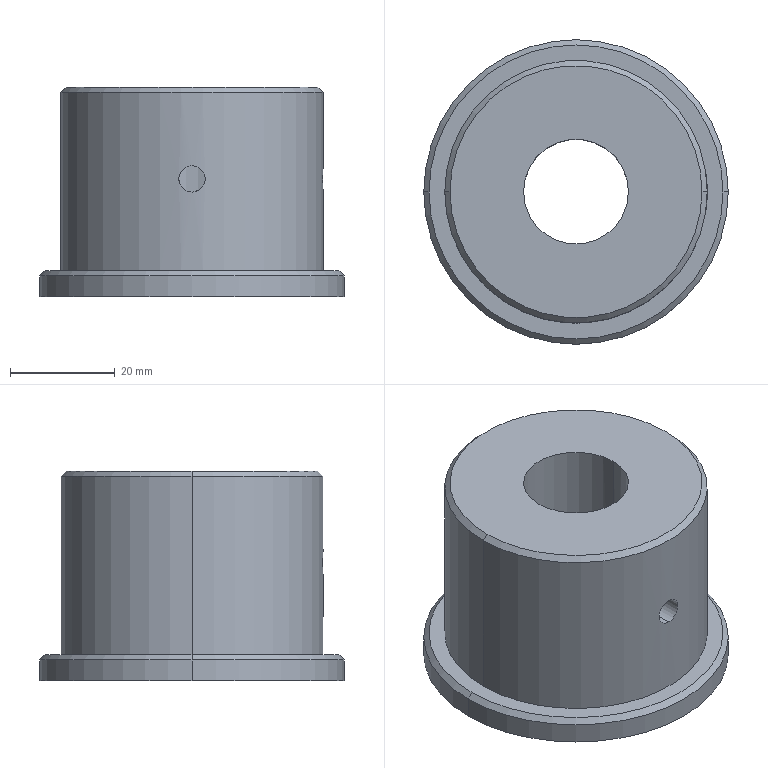Part | SolidWorks | features BaseBody 1 | 1 solid | 17 faces | box 58 x 58 x 40 mm | volume 68608 mm3 | cylinder 10 | cone 4 | plane 3 | commonest cylinder face diameters 5 x4 20 x2 50 x2 58 x2
STEP:
#1=CARTESIAN_POINT('',(24.875,2.5,22.5));
#2=VERTEX_POINT('',#1);
#3=CARTESIAN_POINT('',(25.,0.,20.));
#4=VERTEX_POINT('',#3);
#5=CARTESIAN_POINT('',(24.875,2.5,22.5));
#6=CARTESIAN_POINT('',(24.875,2.5,22.335));
#7=CARTESIAN_POINT('',(24.876,2.484,22.172));
#8=CARTESIAN_POINT('',(24.883,2.42,21.853));
#9=CARTESIAN_POINT('',(24.887,2.372,21.694));
#10=CARTESIAN_POINT('',(24.899,2.247,21.392));
#11=CARTESIAN_POINT('',(24.906,2.17,21.248));
#12=CARTESIAN_POINT('',(24.921,1.989,20.977));
#13=CARTESIAN_POINT('',(24.929,1.884,20.848));
#14=CARTESIAN_POINT('',(24.946,1.653,20.618));
#15=CARTESIAN_POINT('',(24.954,1.528,20.514));
#16=CARTESIAN_POINT('',(24.969,1.255,20.331));
#17=CARTESIAN_POINT('',(24.976,1.109,20.254));
#18=CARTESIAN_POINT('',(24.993,0.6586,20.066));
#19=CARTESIAN_POINT('',(25.,0.3304,20.));
#20=CARTESIAN_POINT('',(25.,0.,20.));
#21=B_SPLINE_CURVE_WITH_KNOTS('',3,(#5,#6,#7,#8,#9,#10,#11,#12,#13,#14,#15,#16,#17,#18,#19,#20),.UNSPECIFIED.,.F.,.F.,(4,2,2,2,2,2,2,4),(0.,0.0004885,0.000977,0.001465,0.001954,0.002442,0.002931,0.003908),.UNSPECIFIED.);
#22=EDGE_CURVE('',#2,#4,#21,.T.);
#23=ORIENTED_EDGE('',*,*,#22,.F.);
#24=CARTESIAN_POINT('',(9.682,2.5,22.5));
#25=VERTEX_POINT('',#24);
#26=CARTESIAN_POINT('',(29.,2.5,22.5));
#27=DIRECTION('',(-1.,0.,0.));
#28=VECTOR('',#27,1000.);
#29=LINE('',#26,#28);
#30=EDGE_CURVE('',#2,#25,#29,.T.);
#31=ORIENTED_EDGE('',*,*,#30,.T.);
#32=CARTESIAN_POINT('',(10.,0.,20.));
#33=VERTEX_POINT('',#32);
#34=CARTESIAN_POINT('',(9.682,2.5,22.5));
#35=CARTESIAN_POINT('',(9.682,2.5,22.334));
#36=CARTESIAN_POINT('',(9.687,2.484,22.171));
#37=CARTESIAN_POINT('',(9.703,2.42,21.851));
#38=CARTESIAN_POINT('',(9.715,2.372,21.692));
#39=CARTESIAN_POINT('',(9.745,2.246,21.39));
#40=CARTESIAN_POINT('',(9.762,2.169,21.247));
#41=CARTESIAN_POINT('',(9.801,1.988,20.975));
#42=CARTESIAN_POINT('',(9.822,1.883,20.848));
#43=CARTESIAN_POINT('',(9.884,1.539,20.503));
#44=CARTESIAN_POINT('',(9.925,1.261,20.317));
#45=CARTESIAN_POINT('',(9.968,0.8108,20.13));
#46=CARTESIAN_POINT('',(9.98,0.653,20.081));
#47=CARTESIAN_POINT('',(9.996,0.3295,20.016));
#48=CARTESIAN_POINT('',(10.,0.1658,20.));
#49=CARTESIAN_POINT('',(10.,0.,20.));
#50=B_SPLINE_CURVE_WITH_KNOTS('',3,(#34,#35,#36,#37,#38,#39,#40,#41,#42,#43,#44,#45,#46,#47,#48,#49),.UNSPECIFIED.,.F.,.F.,(4,2,2,2,2,2,2,4),(0.,0.0004901,0.0009802,0.00147,0.00196,0.002941,0.003431,0.003921),.UNSPECIFIED.);
#51=EDGE_CURVE('',#25,#33,#50,.T.);
#52=ORIENTED_EDGE('',*,*,#51,.T.);
#53=CARTESIAN_POINT('',(9.682,-2.5,22.5));
#54=VERTEX_POINT('',#53);
#55=CARTESIAN_POINT('',(10.,0.,20.));
#56=CARTESIAN_POINT('',(10.,-0.1658,20.));
#57=CARTESIAN_POINT('',(9.996,-0.3287,20.016));
#58=CARTESIAN_POINT('',(9.98,-0.6489,20.08));
#59=CARTESIAN_POINT('',(9.968,-0.808,20.129));
#60=CARTESIAN_POINT('',(9.939,-1.11,20.254));
#61=CARTESIAN_POINT('',(9.922,-1.254,20.331));
#62=CARTESIAN_POINT('',(9.884,-1.525,20.512));
#63=CARTESIAN_POINT('',(9.863,-1.653,20.617));
#64=CARTESIAN_POINT('',(9.801,-1.997,20.961));
#65=CARTESIAN_POINT('',(9.76,-2.183,21.239));
#66=CARTESIAN_POINT('',(9.715,-2.37,21.689));
#67=CARTESIAN_POINT('',(9.703,-2.419,21.847));
#68=CARTESIAN_POINT('',(9.687,-2.484,22.17));
#69=CARTESIAN_POINT('',(9.682,-2.5,22.334));
#70=CARTESIAN_POINT('',(9.682,-2.5,22.5));
#71=B_SPLINE_CURVE_WITH_KNOTS('',3,(#55,#56,#57,#58,#59,#60,#61,#62,#63,#64,#65,#66,#67,#68,#69,#70),.UNSPECIFIED.,.F.,.F.,(4,2,2,2,2,2,2,4),(0.003921,0.004411,0.004901,0.005391,0.005882,0.006862,0.007352,0.007842),.UNSPECIFIED.);
#72=EDGE_CURVE('',#33,#54,#71,.T.);
#73=ORIENTED_EDGE('',*,*,#72,.T.);
#74=CARTESIAN_POINT('',(24.875,-2.5,22.5));
#75=VERTEX_POINT('',#74);
#76=CARTESIAN_POINT('',(29.,-2.5,22.5));
#77=DIRECTION('',(-1.,0.,0.));
#78=VECTOR('',#77,1000.);
#79=LINE('',#76,#78);
#80=EDGE_CURVE('',#75,#54,#79,.T.);
#81=ORIENTED_EDGE('',*,*,#80,.F.);
#82=CARTESIAN_POINT('',(25.,0.,20.));
#83=CARTESIAN_POINT('',(25.,-0.1652,20.));
#84=CARTESIAN_POINT('',(24.998,-0.3276,20.016));
#85=CARTESIAN_POINT('',(24.992,-0.6471,20.08));
#86=CARTESIAN_POINT('',(24.987,-0.8058,20.128));
#87=CARTESIAN_POINT('',(24.976,-1.108,20.253));
#88=CARTESIAN_POINT('',(24.969,-1.252,20.33));
#89=CARTESIAN_POINT('',(24.954,-1.523,20.511));
#90=CARTESIAN_POINT('',(24.946,-1.652,20.616));
#91=CARTESIAN_POINT('',(24.929,-1.882,20.847));
#92=CARTESIAN_POINT('',(24.921,-1.986,20.972));
#93=CARTESIAN_POINT('',(24.906,-2.169,21.245));
#94=CARTESIAN_POINT('',(24.899,-2.246,21.391));
#95=CARTESIAN_POINT('',(24.882,-2.434,21.841));
#96=CARTESIAN_POINT('',(24.875,-2.5,22.17));
#97=CARTESIAN_POINT('',(24.875,-2.5,22.5));
#98=B_SPLINE_CURVE_WITH_KNOTS('',3,(#82,#83,#84,#85,#86,#87,#88,#89,#90,#91,#92,#93,#94,#95,#96,#97),.UNSPECIFIED.,.F.,.F.,(4,2,2,2,2,2,2,4),(0.003908,0.004396,0.004885,0.005373,0.005862,0.00635,0.006839,0.007816),.UNSPECIFIED.);
#99=EDGE_CURVE('',#4,#75,#98,.T.);
#100=ORIENTED_EDGE('',*,*,#99,.F.);
#101=EDGE_LOOP('',(#23,#31,#52,#73,#81,#100));
#102=FACE_OUTER_BOUND('',#101,.T.);
#103=CARTESIAN_POINT('',(29.,0.,22.5));
#104=DIRECTION('',(-1.,0.,0.));
#105=DIRECTION('',(0.,-1.,0.));
#106=AXIS2_PLACEMENT_3D('',#103,#104,#105);
#107=CYLINDRICAL_SURFACE('',#106,2.5);
#108=ADVANCED_FACE('',(#102),#107,.F.);
#109=CARTESIAN_POINT('',(0.,-25.,20.));
#110=VERTEX_POINT('',#109);
#111=CARTESIAN_POINT('',(0.,-25.,25.));
#112=VERTEX_POINT('',#111);
#113=CARTESIAN_POINT('',(0.,-25.,20.));
#114=CARTESIAN_POINT('',(-0.1653,-25.,20.));
#115=CARTESIAN_POINT('',(-0.3277,-24.998,20.016));
#116=CARTESIAN_POINT('',(-0.6473,-24.992,20.08));
#117=CARTESIAN_POINT('',(-0.8062,-24.987,20.128));
#118=CARTESIAN_POINT('',(-1.109,-24.976,20.253));
#119=CARTESIAN_POINT('',(-1.252,-24.969,20.33));
#120=CARTESIAN_POINT('',(-1.524,-24.954,20.512));
#121=CARTESIAN_POINT('',(-1.653,-24.946,20.617));
#122=CARTESIAN_POINT('',(-1.883,-24.929,20.847));
#123=CARTESIAN_POINT('',(-1.986,-24.921,20.973));
#124=CARTESIAN_POINT('',(-2.169,-24.906,21.246));
#125=CARTESIAN_POINT('',(-2.247,-24.899,21.392));
#126=CARTESIAN_POINT('',(-2.372,-24.887,21.693));
#127=CARTESIAN_POINT('',(-2.42,-24.883,21.85));
#128=CARTESIAN_POINT('',(-2.484,-24.876,22.173));
#129=CARTESIAN_POINT('',(-2.5,-24.875,22.335));
#130=CARTESIAN_POINT('',(-2.5,-24.875,22.661));
#131=CARTESIAN_POINT('',(-2.484,-24.876,22.827));
#132=CARTESIAN_POINT('',(-2.42,-24.883,23.148));
#133=CARTESIAN_POINT('',(-2.373,-24.887,23.304));
#134=CARTESIAN_POINT('',(-2.248,-24.899,23.606));
#135=CARTESIAN_POINT('',(-2.17,-24.906,23.753));
#136=CARTESIAN_POINT('',(-1.989,-24.921,24.024));
#137=CARTESIAN_POINT('',(-1.886,-24.929,24.15));
#138=CARTESIAN_POINT('',(-1.652,-24.946,24.383));
#139=CARTESIAN_POINT('',(-1.526,-24.954,24.487));
#140=CARTESIAN_POINT('',(-1.256,-24.969,24.668));
#141=CARTESIAN_POINT('',(-1.11,-24.976,24.746));
#142=CARTESIAN_POINT('',(-0.8069,-24.987,24.872));
#143=CARTESIAN_POINT('',(-0.6511,-24.992,24.919));
#144=CARTESIAN_POINT('',(-0.3307,-24.998,24.983));
#145=CARTESIAN_POINT('',(-0.1653,-25.,25.));
#146=CARTESIAN_POINT('',(0.,-25.,25.));
#147=B_SPLINE_CURVE_WITH_KNOTS('',3,(#113,#114,#115,#116,#117,#118,#119,#120,#121,#122,#123,#124,#125,#126,#127,#128,#129,#130,#131,#132,#133,#134,#135,#136,#137,#138,#139,#140,#141,#142,#143,#144,#145,#146),.UNSPECIFIED.,.F.,.F.,(4,2,2,2,2,2,2,2,2,2,2,2,2,2,2,2,4),(0.,0.0004887,0.0009774,0.001466,0.001955,0.002444,0.002932,0.003421,0.00391,0.004398,0.004887,0.005376,0.005864,0.006353,0.006842,0.007331,0.007819),.UNSPECIFIED.);
#148=EDGE_CURVE('',#110,#112,#147,.T.);
#149=ORIENTED_EDGE('',*,*,#148,.F.);
#150=CARTESIAN_POINT('',(0.,-10.,20.));
#151=VERTEX_POINT('',#150);
#152=CARTESIAN_POINT('',(0.,-29.,20.));
#153=DIRECTION('',(0.,1.,0.));
#154=VECTOR('',#153,1000.);
#155=LINE('',#152,#154);
#156=EDGE_CURVE('',#110,#151,#155,.T.);
#157=ORIENTED_EDGE('',*,*,#156,.T.);
#158=CARTESIAN_POINT('',(0.,-10.,25.));
#159=VERTEX_POINT('',#158);
#160=CARTESIAN_POINT('',(0.,-10.,20.));
#161=CARTESIAN_POINT('',(-0.1658,-10.,20.));
#162=CARTESIAN_POINT('',(-0.3288,-9.996,20.016));
#163=CARTESIAN_POINT('',(-0.6491,-9.98,20.08));
#164=CARTESIAN_POINT('',(-0.8083,-9.968,20.129));
#165=CARTESIAN_POINT('',(-1.111,-9.939,20.254));
#166=CARTESIAN_POINT('',(-1.254,-9.922,20.331));
#167=CARTESIAN_POINT('',(-1.525,-9.884,20.512));
#168=CARTESIAN_POINT('',(-1.653,-9.863,20.618));
#169=CARTESIAN_POINT('',(-1.997,-9.801,20.962));
#170=CARTESIAN_POINT('',(-2.183,-9.76,21.24));
#171=CARTESIAN_POINT('',(-2.371,-9.715,21.69));
#172=CARTESIAN_POINT('',(-2.419,-9.703,21.848));
#173=CARTESIAN_POINT('',(-2.484,-9.687,22.171));
#174=CARTESIAN_POINT('',(-2.5,-9.682,22.334));
#175=CARTESIAN_POINT('',(-2.5,-9.682,22.661));
#176=CARTESIAN_POINT('',(-2.484,-9.687,22.828));
#177=CARTESIAN_POINT('',(-2.42,-9.703,23.149));
#178=CARTESIAN_POINT('',(-2.372,-9.715,23.305));
#179=CARTESIAN_POINT('',(-2.184,-9.759,23.76));
#180=CARTESIAN_POINT('',(-2.,-9.801,24.035));
#181=CARTESIAN_POINT('',(-1.653,-9.863,24.383));
#182=CARTESIAN_POINT('',(-1.528,-9.884,24.486));
#183=CARTESIAN_POINT('',(-1.257,-9.922,24.667));
#184=CARTESIAN_POINT('',(-1.111,-9.939,24.745));
#185=CARTESIAN_POINT('',(-0.8095,-9.968,24.871));
#186=CARTESIAN_POINT('',(-0.6537,-9.98,24.919));
#187=CARTESIAN_POINT('',(-0.3318,-9.996,24.983));
#188=CARTESIAN_POINT('',(-0.1658,-10.,25.));
#189=CARTESIAN_POINT('',(0.,-10.,25.));
#190=B_SPLINE_CURVE_WITH_KNOTS('',3,(#160,#161,#162,#163,#164,#165,#166,#167,#168,#169,#170,#171,#172,#173,#174,#175,#176,#177,#178,#179,#180,#181,#182,#183,#184,#185,#186,#187,#188,#189),.UNSPECIFIED.,.F.,.F.,(4,2,2,2,2,2,2,2,2,2,2,2,2,2,4),(0.,0.0004903,0.0009806,0.001471,0.001961,0.002942,0.003432,0.003922,0.004413,0.004903,0.005884,0.006374,0.006864,0.007355,0.007845),.UNSPECIFIED.);
#191=EDGE_CURVE('',#151,#159,#190,.T.);
#192=ORIENTED_EDGE('',*,*,#191,.T.);
#193=CARTESIAN_POINT('',(0.,-29.,25.));
#194=DIRECTION('',(0.,1.,0.));
#195=VECTOR('',#194,1000.);
#196=LINE('',#193,#195);
#197=EDGE_CURVE('',#112,#159,#196,.T.);
#198=ORIENTED_EDGE('',*,*,#197,.F.);
#199=EDGE_LOOP('',(#149,#157,#192,#198));
#200=FACE_OUTER_BOUND('',#199,.T.);
#201=CARTESIAN_POINT('',(0.,-29.,22.5));
#202=DIRECTION('',(0.,1.,0.));
#203=DIRECTION('',(0.,0.,1.));
#204=AXIS2_PLACEMENT_3D('',#201,#202,#203);
#205=CYLINDRICAL_SURFACE('',#204,2.5);
#206=ADVANCED_FACE('',(#200),#205,.F.);
#207=CARTESIAN_POINT('',(24.,0.,40.));
#208=VERTEX_POINT('',#207);
#209=CARTESIAN_POINT('',(-24.,0.,40.));
#210=VERTEX_POINT('',#209);
#211=CARTESIAN_POINT('',(0.,0.,40.));
#212=DIRECTION('',(0.,0.,1.));
#213=DIRECTION('',(1.,0.,0.));
#214=AXIS2_PLACEMENT_3D('',#211,#212,#213);
#215=CIRCLE('',#214,24.);
#216=EDGE_CURVE('',#208,#210,#215,.T.);
#217=ORIENTED_EDGE('',*,*,#216,.F.);
#218=CARTESIAN_POINT('',(25.,0.,39.));
#219=VERTEX_POINT('',#218);
#220=CARTESIAN_POINT('',(24.,0.,40.));
#221=DIRECTION('',(0.7071,0.,-0.7071));
#222=VECTOR('',#221,1000.);
#223=LINE('',#220,#222);
#224=EDGE_CURVE('',#208,#219,#223,.T.);
#225=ORIENTED_EDGE('',*,*,#224,.T.);
#226=CARTESIAN_POINT('',(-25.,0.,39.));
#227=VERTEX_POINT('',#226);
#228=CARTESIAN_POINT('',(0.,0.,39.));
#229=DIRECTION('',(0.,0.,-1.));
#230=DIRECTION('',(1.,0.,0.));
#231=AXIS2_PLACEMENT_3D('',#228,#229,#230);
#232=CIRCLE('',#231,25.);
#233=EDGE_CURVE('',#227,#219,#232,.T.);
#234=ORIENTED_EDGE('',*,*,#233,.F.);
#235=CARTESIAN_POINT('',(-24.,0.,40.));
#236=DIRECTION('',(-0.7071,0.,-0.7071));
#237=VECTOR('',#236,1000.);
#238=LINE('',#235,#237);
#239=EDGE_CURVE('',#210,#227,#238,.T.);
#240=ORIENTED_EDGE('',*,*,#239,.F.);
#241=EDGE_LOOP('',(#217,#225,#234,#240));
#242=FACE_OUTER_BOUND('',#241,.T.);
#243=CARTESIAN_POINT('',(0.,0.,40.));
#244=DIRECTION('',(0.,0.,-1.));
#245=DIRECTION('',(-1.,0.,0.));
#246=AXIS2_PLACEMENT_3D('',#243,#244,#245);
#247=CONICAL_SURFACE('',#246,24.,0.7854);
#248=ADVANCED_FACE('',(#242),#247,.T.);
#249=CARTESIAN_POINT('',(28.,0.,5.));
#250=VERTEX_POINT('',#249);
#251=CARTESIAN_POINT('',(-28.,0.,5.));
#252=VERTEX_POINT('',#251);
#253=CARTESIAN_POINT('',(0.,0.,5.));
#254=DIRECTION('',(0.,0.,1.));
#255=DIRECTION('',(1.,0.,0.));
#256=AXIS2_PLACEMENT_3D('',#253,#254,#255);
#257=CIRCLE('',#256,28.);
#258=EDGE_CURVE('',#250,#252,#257,.T.);
#259=ORIENTED_EDGE('',*,*,#258,.F.);
#260=CARTESIAN_POINT('',(29.,0.,4.));
#261=VERTEX_POINT('',#260);
#262=CARTESIAN_POINT('',(28.,0.,5.));
#263=DIRECTION('',(0.7071,0.,-0.7071));
#264=VECTOR('',#263,1000.);
#265=LINE('',#262,#264);
#266=EDGE_CURVE('',#250,#261,#265,.T.);
#267=ORIENTED_EDGE('',*,*,#266,.T.);
#268=CARTESIAN_POINT('',(-29.,0.,4.));
#269=VERTEX_POINT('',#268);
#270=CARTESIAN_POINT('',(0.,0.,4.));
#271=DIRECTION('',(0.,0.,-1.));
#272=DIRECTION('',(1.,0.,0.));
#273=AXIS2_PLACEMENT_3D('',#270,#271,#272);
#274=CIRCLE('',#273,29.);
#275=EDGE_CURVE('',#269,#261,#274,.T.);
#276=ORIENTED_EDGE('',*,*,#275,.F.);
#277=CARTESIAN_POINT('',(-28.,0.,5.));
#278=DIRECTION('',(-0.7071,0.,-0.7071));
#279=VECTOR('',#278,1000.);
#280=LINE('',#277,#279);
#281=EDGE_CURVE('',#252,#269,#280,.T.);
#282=ORIENTED_EDGE('',*,*,#281,.F.);
#283=EDGE_LOOP('',(#259,#267,#276,#282));
#284=FACE_OUTER_BOUND('',#283,.T.);
#285=CARTESIAN_POINT('',(0.,0.,5.));
#286=DIRECTION('',(0.,0.,-1.));
#287=DIRECTION('',(-1.,0.,0.));
#288=AXIS2_PLACEMENT_3D('',#285,#286,#287);
#289=CONICAL_SURFACE('',#288,28.,0.7854);
#290=ADVANCED_FACE('',(#284),#289,.T.);
#291=CARTESIAN_POINT('',(0.,-10.,25.));
#292=CARTESIAN_POINT('',(0.1658,-10.,25.));
#293=CARTESIAN_POINT('',(0.3288,-9.996,24.984));
#294=CARTESIAN_POINT('',(0.6491,-9.98,24.92));
#295=CARTESIAN_POINT('',(0.8083,-9.968,24.871));
#296=CARTESIAN_POINT('',(1.111,-9.939,24.746));
#297=CARTESIAN_POINT('',(1.254,-9.922,24.669));
#298=CARTESIAN_POINT('',(1.525,-9.884,24.488));
#299=CARTESIAN_POINT('',(1.653,-9.863,24.382));
#300=CARTESIAN_POINT('',(1.997,-9.801,24.038));
#301=CARTESIAN_POINT('',(2.183,-9.76,23.76));
#302=CARTESIAN_POINT('',(2.371,-9.715,23.31));
#303=CARTESIAN_POINT('',(2.419,-9.703,23.152));
#304=CARTESIAN_POINT('',(2.484,-9.687,22.829));
#305=CARTESIAN_POINT('',(2.5,-9.682,22.666));
#306=CARTESIAN_POINT('',(2.5,-9.682,22.339));
#307=CARTESIAN_POINT('',(2.484,-9.687,22.172));
#308=CARTESIAN_POINT('',(2.42,-9.703,21.851));
#309=CARTESIAN_POINT('',(2.372,-9.715,21.695));
#310=CARTESIAN_POINT('',(2.184,-9.759,21.24));
#311=CARTESIAN_POINT('',(2.,-9.801,20.965));
#312=CARTESIAN_POINT('',(1.653,-9.863,20.617));
#313=CARTESIAN_POINT('',(1.528,-9.884,20.514));
#314=CARTESIAN_POINT('',(1.257,-9.922,20.333));
#315=CARTESIAN_POINT('',(1.111,-9.939,20.255));
#316=CARTESIAN_POINT('',(0.8095,-9.968,20.129));
#317=CARTESIAN_POINT('',(0.6537,-9.98,20.081));
#318=CARTESIAN_POINT('',(0.3318,-9.996,20.017));
#319=CARTESIAN_POINT('',(0.1658,-10.,20.));
#320=CARTESIAN_POINT('',(0.,-10.,20.));
#321=B_SPLINE_CURVE_WITH_KNOTS('',3,(#291,#292,#293,#294,#295,#296,#297,#298,#299,#300,#301,#302,#303,#304,#305,#306,#307,#308,#309,#310,#311,#312,#313,#314,#315,#316,#317,#318,#319,#320),.UNSPECIFIED.,.F.,.F.,(4,2,2,2,2,2,2,2,2,2,2,2,2,2,4),(0.007845,0.008335,0.008826,0.009316,0.009806,0.01079,0.01128,0.01177,0.01226,0.01275,0.01373,0.01422,0.01471,0.0152,0.01569),.UNSPECIFIED.);
#322=EDGE_CURVE('',#159,#151,#321,.T.);
#323=ORIENTED_EDGE('',*,*,#322,.F.);
#324=ORIENTED_EDGE('',*,*,#191,.F.);
#325=EDGE_LOOP('',(#323,#324));
#326=FACE_BOUND('',#325,.T.);
#327=CARTESIAN_POINT('',(-10.,0.,40.));
#328=VERTEX_POINT('',#327);
#329=CARTESIAN_POINT('',(10.,0.,40.));
#330=VERTEX_POINT('',#329);
#331=CARTESIAN_POINT('',(0.,0.,40.));
#332=DIRECTION('',(0.,0.,1.));
#333=DIRECTION('',(1.,0.,0.));
#334=AXIS2_PLACEMENT_3D('',#331,#332,#333);
#335=CIRCLE('',#334,10.);
#336=EDGE_CURVE('',#328,#330,#335,.T.);
#337=ORIENTED_EDGE('',*,*,#336,.T.);
#338=CARTESIAN_POINT('',(10.,0.,25.));
#339=VERTEX_POINT('',#338);
#340=CARTESIAN_POINT('',(10.,0.,40.));
#341=DIRECTION('',(0.,0.,-1.));
#342=VECTOR('',#341,1000.);
#343=LINE('',#340,#342);
#344=EDGE_CURVE('',#330,#339,#343,.T.);
#345=ORIENTED_EDGE('',*,*,#344,.T.);
#346=CARTESIAN_POINT('',(9.682,-2.5,22.5));
#347=CARTESIAN_POINT('',(9.682,-2.5,22.666));
#348=CARTESIAN_POINT('',(9.687,-2.484,22.829));
#349=CARTESIAN_POINT('',(9.703,-2.42,23.149));
#350=CARTESIAN_POINT('',(9.715,-2.372,23.308));
#351=CARTESIAN_POINT('',(9.745,-2.246,23.61));
#352=CARTESIAN_POINT('',(9.762,-2.169,23.753));
#353=CARTESIAN_POINT('',(9.801,-1.988,24.025));
#354=CARTESIAN_POINT('',(9.822,-1.883,24.152));
#355=CARTESIAN_POINT('',(9.884,-1.539,24.497));
#356=CARTESIAN_POINT('',(9.925,-1.261,24.683));
#357=CARTESIAN_POINT('',(9.968,-0.8108,24.87));
#358=CARTESIAN_POINT('',(9.98,-0.653,24.919));
#359=CARTESIAN_POINT('',(9.996,-0.3295,24.984));
#360=CARTESIAN_POINT('',(10.,-0.1658,25.));
#361=CARTESIAN_POINT('',(10.,0.,25.));
#362=B_SPLINE_CURVE_WITH_KNOTS('',3,(#346,#347,#348,#349,#350,#351,#352,#353,#354,#355,#356,#357,#358,#359,#360,#361),.UNSPECIFIED.,.F.,.F.,(4,2,2,2,2,2,2,4),(0.007842,0.008332,0.008822,0.009313,0.009803,0.01078,0.01127,0.01176),.UNSPECIFIED.);
#363=EDGE_CURVE('',#54,#339,#362,.T.);
#364=ORIENTED_EDGE('',*,*,#363,.F.);
#365=ORIENTED_EDGE('',*,*,#72,.F.);
#366=CARTESIAN_POINT('',(10.,0.,0.));
#367=VERTEX_POINT('',#366);
#368=CARTESIAN_POINT('',(10.,0.,40.));
#369=DIRECTION('',(0.,0.,-1.));
#370=VECTOR('',#369,1000.);
#371=LINE('',#368,#370);
#372=EDGE_CURVE('',#33,#367,#371,.T.);
#373=ORIENTED_EDGE('',*,*,#372,.T.);
#374=CARTESIAN_POINT('',(-10.,0.,0.));
#375=VERTEX_POINT('',#374);
#376=CARTESIAN_POINT('',(0.,0.,0.));
#377=DIRECTION('',(0.,0.,1.));
#378=DIRECTION('',(1.,0.,0.));
#379=AXIS2_PLACEMENT_3D('',#376,#377,#378);
#380=CIRCLE('',#379,10.);
#381=EDGE_CURVE('',#375,#367,#380,.T.);
#382=ORIENTED_EDGE('',*,*,#381,.F.);
#383=CARTESIAN_POINT('',(-10.,0.,40.));
#384=DIRECTION('',(0.,0.,-1.));
#385=VECTOR('',#384,1000.);
#386=LINE('',#383,#385);
#387=EDGE_CURVE('',#328,#375,#386,.T.);
#388=ORIENTED_EDGE('',*,*,#387,.F.);
#389=EDGE_LOOP('',(#337,#345,#364,#365,#373,#382,#388));
#390=FACE_OUTER_BOUND('',#389,.T.);
#391=CARTESIAN_POINT('',(0.,0.,40.));
#392=DIRECTION('',(0.,0.,-1.));
#393=DIRECTION('',(-1.,0.,0.));
#394=AXIS2_PLACEMENT_3D('',#391,#392,#393);
#395=CYLINDRICAL_SURFACE('',#394,10.);
#396=ADVANCED_FACE('',(#326,#390),#395,.F.);
#397=ORIENTED_EDGE('',*,*,#233,.T.);
#398=CARTESIAN_POINT('',(25.,0.,25.));
#399=VERTEX_POINT('',#398);
#400=CARTESIAN_POINT('',(25.,0.,40.));
#401=DIRECTION('',(0.,0.,-1.));
#402=VECTOR('',#401,1000.);
#403=LINE('',#400,#402);
#404=EDGE_CURVE('',#219,#399,#403,.T.);
#405=ORIENTED_EDGE('',*,*,#404,.T.);
#406=CARTESIAN_POINT('',(25.,0.,25.));
#407=CARTESIAN_POINT('',(25.,0.1652,25.));
#408=CARTESIAN_POINT('',(24.998,0.3276,24.984));
#409=CARTESIAN_POINT('',(24.992,0.6471,24.92));
#410=CARTESIAN_POINT('',(24.987,0.8058,24.872));
#411=CARTESIAN_POINT('',(24.976,1.108,24.747));
#412=CARTESIAN_POINT('',(24.969,1.252,24.67));
#413=CARTESIAN_POINT('',(24.954,1.523,24.489));
#414=CARTESIAN_POINT('',(24.946,1.652,24.384));
#415=CARTESIAN_POINT('',(24.929,1.882,24.153));
#416=CARTESIAN_POINT('',(24.921,1.986,24.028));
#417=CARTESIAN_POINT('',(24.906,2.169,23.755));
#418=CARTESIAN_POINT('',(24.899,2.246,23.609));
#419=CARTESIAN_POINT('',(24.882,2.434,23.159));
#420=CARTESIAN_POINT('',(24.875,2.5,22.83));
#421=CARTESIAN_POINT('',(24.875,2.5,22.5));
#422=B_SPLINE_CURVE_WITH_KNOTS('',3,(#406,#407,#408,#409,#410,#411,#412,#413,#414,#415,#416,#417,#418,#419,#420,#421),.UNSPECIFIED.,.F.,.F.,(4,2,2,2,2,2,2,4),(0.01172,0.01221,0.0127,0.01319,0.01368,0.01417,0.01465,0.01563),.UNSPECIFIED.);
#423=EDGE_CURVE('',#399,#2,#422,.T.);
#424=ORIENTED_EDGE('',*,*,#423,.T.);
#425=ORIENTED_EDGE('',*,*,#22,.T.);
#426=CARTESIAN_POINT('',(25.,0.,5.));
#427=VERTEX_POINT('',#426);
#428=CARTESIAN_POINT('',(25.,0.,40.));
#429=DIRECTION('',(0.,0.,-1.));
#430=VECTOR('',#429,1000.);
#431=LINE('',#428,#430);
#432=EDGE_CURVE('',#4,#427,#431,.T.);
#433=ORIENTED_EDGE('',*,*,#432,.T.);
#434=CARTESIAN_POINT('',(-25.,0.,5.));
#435=VERTEX_POINT('',#434);
#436=CARTESIAN_POINT('',(0.,0.,5.));
#437=DIRECTION('',(0.,0.,1.));
#438=DIRECTION('',(1.,0.,0.));
#439=AXIS2_PLACEMENT_3D('',#436,#437,#438);
#440=CIRCLE('',#439,25.);
#441=EDGE_CURVE('',#427,#435,#440,.T.);
#442=ORIENTED_EDGE('',*,*,#441,.T.);
#443=CARTESIAN_POINT('',(-25.,0.,40.));
#444=DIRECTION('',(0.,0.,-1.));
#445=VECTOR('',#444,1000.);
#446=LINE('',#443,#445);
#447=EDGE_CURVE('',#227,#435,#446,.T.);
#448=ORIENTED_EDGE('',*,*,#447,.F.);
#449=EDGE_LOOP('',(#397,#405,#424,#425,#433,#442,#448));
#450=FACE_OUTER_BOUND('',#449,.T.);
#451=CARTESIAN_POINT('',(0.,0.,40.));
#452=DIRECTION('',(0.,0.,-1.));
#453=DIRECTION('',(-1.,0.,0.));
#454=AXIS2_PLACEMENT_3D('',#451,#452,#453);
#455=CYLINDRICAL_SURFACE('',#454,25.);
#456=ADVANCED_FACE('',(#450),#455,.T.);
#457=ORIENTED_EDGE('',*,*,#275,.T.);
#458=CARTESIAN_POINT('',(29.,0.,0.));
#459=VERTEX_POINT('',#458);
#460=CARTESIAN_POINT('',(29.,0.,5.));
#461=DIRECTION('',(0.,0.,-1.));
#462=VECTOR('',#461,1000.);
#463=LINE('',#460,#462);
#464=EDGE_CURVE('',#261,#459,#463,.T.);
#465=ORIENTED_EDGE('',*,*,#464,.T.);
#466=CARTESIAN_POINT('',(-29.,0.,0.));
#467=VERTEX_POINT('',#466);
#468=CARTESIAN_POINT('',(0.,0.,0.));
#469=DIRECTION('',(0.,0.,1.));
#470=DIRECTION('',(1.,0.,0.));
#471=AXIS2_PLACEMENT_3D('',#468,#469,#470);
#472=CIRCLE('',#471,29.);
#473=EDGE_CURVE('',#459,#467,#472,.T.);
#474=ORIENTED_EDGE('',*,*,#473,.T.);
#475=CARTESIAN_POINT('',(-29.,0.,5.));
#476=DIRECTION('',(0.,0.,-1.));
#477=VECTOR('',#476,1000.);
#478=LINE('',#475,#477);
#479=EDGE_CURVE('',#269,#467,#478,.T.);
#480=ORIENTED_EDGE('',*,*,#479,.F.);
#481=EDGE_LOOP('',(#457,#465,#474,#480));
#482=FACE_OUTER_BOUND('',#481,.T.);
#483=CARTESIAN_POINT('',(0.,0.,5.));
#484=DIRECTION('',(0.,0.,-1.));
#485=DIRECTION('',(-1.,0.,0.));
#486=AXIS2_PLACEMENT_3D('',#483,#484,#485);
#487=CYLINDRICAL_SURFACE('',#486,29.);
#488=ADVANCED_FACE('',(#482),#487,.T.);
#489=ORIENTED_EDGE('',*,*,#336,.F.);
#490=CARTESIAN_POINT('',(0.,0.,40.));
#491=DIRECTION('',(0.,0.,1.));
#492=DIRECTION('',(1.,0.,0.));
#493=AXIS2_PLACEMENT_3D('',#490,#491,#492);
#494=CIRCLE('',#493,10.);
#495=EDGE_CURVE('',#330,#328,#494,.T.);
#496=ORIENTED_EDGE('',*,*,#495,.F.);
#497=EDGE_LOOP('',(#489,#496));
#498=FACE_BOUND('',#497,.T.);
#499=CARTESIAN_POINT('',(0.,0.,40.));
#500=DIRECTION('',(0.,0.,1.));
#501=DIRECTION('',(1.,0.,0.));
#502=AXIS2_PLACEMENT_3D('',#499,#500,#501);
#503=CIRCLE('',#502,24.);
#504=EDGE_CURVE('',#210,#208,#503,.T.);
#505=ORIENTED_EDGE('',*,*,#504,.T.);
#506=ORIENTED_EDGE('',*,*,#216,.T.);
#507=EDGE_LOOP('',(#505,#506));
#508=FACE_OUTER_BOUND('',#507,.T.);
#509=CARTESIAN_POINT('',(0.,0.,40.));
#510=DIRECTION('',(0.,0.,1.));
#511=DIRECTION('',(1.,0.,0.));
#512=AXIS2_PLACEMENT_3D('',#509,#510,#511);
#513=PLANE('',#512);
#514=ADVANCED_FACE('',(#498,#508),#513,.T.);
#515=ORIENTED_EDGE('',*,*,#381,.T.);
#516=CARTESIAN_POINT('',(0.,0.,0.));
#517=DIRECTION('',(0.,0.,1.));
#518=DIRECTION('',(1.,0.,0.));
#519=AXIS2_PLACEMENT_3D('',#516,#517,#518);
#520=CIRCLE('',#519,10.);
#521=EDGE_CURVE('',#367,#375,#520,.T.);
#522=ORIENTED_EDGE('',*,*,#521,.T.);
#523=EDGE_LOOP('',(#515,#522));
#524=FACE_BOUND('',#523,.T.);
#525=CARTESIAN_POINT('',(0.,0.,0.));
#526=DIRECTION('',(0.,0.,1.));
#527=DIRECTION('',(1.,0.,0.));
#528=AXIS2_PLACEMENT_3D('',#525,#526,#527);
#529=CIRCLE('',#528,29.);
#530=EDGE_CURVE('',#467,#459,#529,.T.);
#531=ORIENTED_EDGE('',*,*,#530,.F.);
#532=ORIENTED_EDGE('',*,*,#473,.F.);
#533=EDGE_LOOP('',(#531,#532));
#534=FACE_OUTER_BOUND('',#533,.T.);
#535=CARTESIAN_POINT('',(0.,0.,0.));
#536=DIRECTION('',(0.,0.,1.));
#537=DIRECTION('',(1.,0.,0.));
#538=AXIS2_PLACEMENT_3D('',#535,#536,#537);
#539=PLANE('',#538);
#540=ADVANCED_FACE('',(#524,#534),#539,.F.);
#541=CARTESIAN_POINT('',(0.,0.,5.));
#542=DIRECTION('',(0.,0.,1.));
#543=DIRECTION('',(1.,0.,0.));
#544=AXIS2_PLACEMENT_3D('',#541,#542,#543);
#545=CIRCLE('',#544,25.);
#546=EDGE_CURVE('',#435,#427,#545,.T.);
#547=ORIENTED_EDGE('',*,*,#546,.F.);
#548=ORIENTED_EDGE('',*,*,#441,.F.);
#549=EDGE_LOOP('',(#547,#548));
#550=FACE_BOUND('',#549,.T.);
#551=CARTESIAN_POINT('',(0.,0.,5.));
#552=DIRECTION('',(0.,0.,1.));
#553=DIRECTION('',(1.,0.,0.));
#554=AXIS2_PLACEMENT_3D('',#551,#552,#553);
#555=CIRCLE('',#554,28.);
#556=EDGE_CURVE('',#252,#250,#555,.T.);
#557=ORIENTED_EDGE('',*,*,#556,.T.);
#558=ORIENTED_EDGE('',*,*,#258,.T.);
#559=EDGE_LOOP('',(#557,#558));
#560=FACE_OUTER_BOUND('',#559,.T.);
#561=CARTESIAN_POINT('',(0.,0.,5.));
#562=DIRECTION('',(0.,0.,1.));
#563=DIRECTION('',(1.,0.,0.));
#564=AXIS2_PLACEMENT_3D('',#561,#562,#563);
#565=PLANE('',#564);
#566=ADVANCED_FACE('',(#550,#560),#565,.T.);
#567=ORIENTED_EDGE('',*,*,#464,.F.);
#568=CARTESIAN_POINT('',(0.,0.,4.));
#569=DIRECTION('',(0.,0.,-1.));
#570=DIRECTION('',(1.,0.,0.));
#571=AXIS2_PLACEMENT_3D('',#568,#569,#570);
#572=CIRCLE('',#571,29.);
#573=EDGE_CURVE('',#261,#269,#572,.T.);
#574=ORIENTED_EDGE('',*,*,#573,.T.);
#575=ORIENTED_EDGE('',*,*,#479,.T.);
#576=ORIENTED_EDGE('',*,*,#530,.T.);
#577=EDGE_LOOP('',(#567,#574,#575,#576));
#578=FACE_OUTER_BOUND('',#577,.T.);
#579=CARTESIAN_POINT('',(0.,0.,5.));
#580=DIRECTION('',(0.,0.,-1.));
#581=DIRECTION('',(-1.,0.,0.));
#582=AXIS2_PLACEMENT_3D('',#579,#580,#581);
#583=CYLINDRICAL_SURFACE('',#582,29.);
#584=ADVANCED_FACE('',(#578),#583,.T.);
#585=ORIENTED_EDGE('',*,*,#404,.F.);
#586=CARTESIAN_POINT('',(0.,0.,39.));
#587=DIRECTION('',(0.,0.,-1.));
#588=DIRECTION('',(1.,0.,0.));
#589=AXIS2_PLACEMENT_3D('',#586,#587,#588);
#590=CIRCLE('',#589,25.);
#591=EDGE_CURVE('',#219,#227,#590,.T.);
#592=ORIENTED_EDGE('',*,*,#591,.T.);
#593=ORIENTED_EDGE('',*,*,#447,.T.);
#594=ORIENTED_EDGE('',*,*,#546,.T.);
#595=ORIENTED_EDGE('',*,*,#432,.F.);
#596=ORIENTED_EDGE('',*,*,#99,.T.);
#597=CARTESIAN_POINT('',(24.875,-2.5,22.5));
#598=CARTESIAN_POINT('',(24.875,-2.5,22.665));
#599=CARTESIAN_POINT('',(24.876,-2.484,22.828));
#600=CARTESIAN_POINT('',(24.883,-2.42,23.147));
#601=CARTESIAN_POINT('',(24.887,-2.372,23.306));
#602=CARTESIAN_POINT('',(24.899,-2.247,23.608));
#603=CARTESIAN_POINT('',(24.906,-2.17,23.752));
#604=CARTESIAN_POINT('',(24.921,-1.989,24.023));
#605=CARTESIAN_POINT('',(24.929,-1.884,24.152));
#606=CARTESIAN_POINT('',(24.946,-1.653,24.382));
#607=CARTESIAN_POINT('',(24.954,-1.528,24.486));
#608=CARTESIAN_POINT('',(24.969,-1.255,24.669));
#609=CARTESIAN_POINT('',(24.976,-1.109,24.746));
#610=CARTESIAN_POINT('',(24.993,-0.6586,24.934));
#611=CARTESIAN_POINT('',(25.,-0.3304,25.));
#612=CARTESIAN_POINT('',(25.,0.,25.));
#613=B_SPLINE_CURVE_WITH_KNOTS('',3,(#597,#598,#599,#600,#601,#602,#603,#604,#605,#606,#607,#608,#609,#610,#611,#612),.UNSPECIFIED.,.F.,.F.,(4,2,2,2,2,2,2,4),(0.007816,0.008304,0.008793,0.009281,0.00977,0.01026,0.01075,0.01172),.UNSPECIFIED.);
#614=EDGE_CURVE('',#75,#399,#613,.T.);
#615=ORIENTED_EDGE('',*,*,#614,.T.);
#616=EDGE_LOOP('',(#585,#592,#593,#594,#595,#596,#615));
#617=FACE_OUTER_BOUND('',#616,.T.);
#618=CARTESIAN_POINT('',(0.,-25.,25.));
#619=CARTESIAN_POINT('',(0.1653,-25.,25.));
#620=CARTESIAN_POINT('',(0.3277,-24.998,24.984));
#621=CARTESIAN_POINT('',(0.6473,-24.992,24.92));
#622=CARTESIAN_POINT('',(0.8062,-24.987,24.872));
#623=CARTESIAN_POINT('',(1.109,-24.976,24.747));
#624=CARTESIAN_POINT('',(1.252,-24.969,24.67));
#625=CARTESIAN_POINT('',(1.524,-24.954,24.488));
#626=CARTESIAN_POINT('',(1.653,-24.946,24.383));
#627=CARTESIAN_POINT('',(1.883,-24.929,24.153));
#628=CARTESIAN_POINT('',(1.986,-24.921,24.027));
#629=CARTESIAN_POINT('',(2.169,-24.906,23.754));
#630=CARTESIAN_POINT('',(2.247,-24.899,23.608));
#631=CARTESIAN_POINT('',(2.372,-24.887,23.307));
#632=CARTESIAN_POINT('',(2.42,-24.883,23.15));
#633=CARTESIAN_POINT('',(2.484,-24.876,22.827));
#634=CARTESIAN_POINT('',(2.5,-24.875,22.665));
#635=CARTESIAN_POINT('',(2.5,-24.875,22.339));
#636=CARTESIAN_POINT('',(2.484,-24.876,22.173));
#637=CARTESIAN_POINT('',(2.42,-24.883,21.852));
#638=CARTESIAN_POINT('',(2.373,-24.887,21.696));
#639=CARTESIAN_POINT('',(2.248,-24.899,21.394));
#640=CARTESIAN_POINT('',(2.17,-24.906,21.247));
#641=CARTESIAN_POINT('',(1.989,-24.921,20.976));
#642=CARTESIAN_POINT('',(1.886,-24.929,20.85));
#643=CARTESIAN_POINT('',(1.652,-24.946,20.617));
#644=CARTESIAN_POINT('',(1.526,-24.954,20.513));
#645=CARTESIAN_POINT('',(1.256,-24.969,20.332));
#646=CARTESIAN_POINT('',(1.11,-24.976,20.254));
#647=CARTESIAN_POINT('',(0.8069,-24.987,20.128));
#648=CARTESIAN_POINT('',(0.6511,-24.992,20.081));
#649=CARTESIAN_POINT('',(0.3307,-24.998,20.017));
#650=CARTESIAN_POINT('',(0.1653,-25.,20.));
#651=CARTESIAN_POINT('',(0.,-25.,20.));
#652=B_SPLINE_CURVE_WITH_KNOTS('',3,(#618,#619,#620,#621,#622,#623,#624,#625,#626,#627,#628,#629,#630,#631,#632,#633,#634,#635,#636,#637,#638,#639,#640,#641,#642,#643,#644,#645,#646,#647,#648,#649,#650,#651),.UNSPECIFIED.,.F.,.F.,(4,2,2,2,2,2,2,2,2,2,2,2,2,2,2,2,4),(0.007819,0.008308,0.008797,0.009285,0.009774,0.01026,0.01075,0.01124,0.01173,0.01222,0.01271,0.0132,0.01368,0.01417,0.01466,0.01515,0.01564),.UNSPECIFIED.);
#653=EDGE_CURVE('',#112,#110,#652,.T.);
#654=ORIENTED_EDGE('',*,*,#653,.T.);
#655=ORIENTED_EDGE('',*,*,#148,.T.);
#656=EDGE_LOOP('',(#654,#655));
#657=FACE_BOUND('',#656,.T.);
#658=CARTESIAN_POINT('',(0.,0.,40.));
#659=DIRECTION('',(0.,0.,-1.));
#660=DIRECTION('',(-1.,0.,0.));
#661=AXIS2_PLACEMENT_3D('',#658,#659,#660);
#662=CYLINDRICAL_SURFACE('',#661,25.);
#663=ADVANCED_FACE('',(#617,#657),#662,.T.);
#664=ORIENTED_EDGE('',*,*,#344,.F.);
#665=ORIENTED_EDGE('',*,*,#495,.T.);
#666=ORIENTED_EDGE('',*,*,#387,.T.);
#667=ORIENTED_EDGE('',*,*,#521,.F.);
#668=ORIENTED_EDGE('',*,*,#372,.F.);
#669=ORIENTED_EDGE('',*,*,#51,.F.);
#670=CARTESIAN_POINT('',(10.,0.,25.));
#671=CARTESIAN_POINT('',(10.,0.1658,25.));
#672=CARTESIAN_POINT('',(9.996,0.3287,24.984));
#673=CARTESIAN_POINT('',(9.98,0.6489,24.92));
#674=CARTESIAN_POINT('',(9.968,0.808,24.871));
#675=CARTESIAN_POINT('',(9.939,1.11,24.746));
#676=CARTESIAN_POINT('',(9.922,1.254,24.669));
#677=CARTESIAN_POINT('',(9.884,1.525,24.488));
#678=CARTESIAN_POINT('',(9.863,1.653,24.383));
#679=CARTESIAN_POINT('',(9.801,1.997,24.039));
#680=CARTESIAN_POINT('',(9.76,2.183,23.761));
#681=CARTESIAN_POINT('',(9.715,2.37,23.311));
#682=CARTESIAN_POINT('',(9.703,2.419,23.153));
#683=CARTESIAN_POINT('',(9.687,2.484,22.83));
#684=CARTESIAN_POINT('',(9.682,2.5,22.666));
#685=CARTESIAN_POINT('',(9.682,2.5,22.5));
#686=B_SPLINE_CURVE_WITH_KNOTS('',3,(#670,#671,#672,#673,#674,#675,#676,#677,#678,#679,#680,#681,#682,#683,#684,#685),.UNSPECIFIED.,.F.,.F.,(4,2,2,2,2,2,2,4),(0.01176,0.01225,0.01274,0.01323,0.01372,0.0147,0.01519,0.01568),.UNSPECIFIED.);
#687=EDGE_CURVE('',#339,#25,#686,.T.);
#688=ORIENTED_EDGE('',*,*,#687,.F.);
#689=EDGE_LOOP('',(#664,#665,#666,#667,#668,#669,#688));
#690=FACE_OUTER_BOUND('',#689,.T.);
#691=CARTESIAN_POINT('',(0.,0.,40.));
#692=DIRECTION('',(0.,0.,-1.));
#693=DIRECTION('',(-1.,0.,0.));
#694=AXIS2_PLACEMENT_3D('',#691,#692,#693);
#695=CYLINDRICAL_SURFACE('',#694,10.);
#696=ADVANCED_FACE('',(#690),#695,.F.);
#697=ORIENTED_EDGE('',*,*,#266,.F.);
#698=ORIENTED_EDGE('',*,*,#556,.F.);
#699=ORIENTED_EDGE('',*,*,#281,.T.);
#700=ORIENTED_EDGE('',*,*,#573,.F.);
#701=EDGE_LOOP('',(#697,#698,#699,#700));
#702=FACE_OUTER_BOUND('',#701,.T.);
#703=CARTESIAN_POINT('',(0.,0.,5.));
#704=DIRECTION('',(0.,0.,-1.));
#705=DIRECTION('',(-1.,0.,0.));
#706=AXIS2_PLACEMENT_3D('',#703,#704,#705);
#707=CONICAL_SURFACE('',#706,28.,0.7854);
#708=ADVANCED_FACE('',(#702),#707,.T.);
#709=ORIENTED_EDGE('',*,*,#224,.F.);
#710=ORIENTED_EDGE('',*,*,#504,.F.);
#711=ORIENTED_EDGE('',*,*,#239,.T.);
#712=ORIENTED_EDGE('',*,*,#591,.F.);
#713=EDGE_LOOP('',(#709,#710,#711,#712));
#714=FACE_OUTER_BOUND('',#713,.T.);
#715=CARTESIAN_POINT('',(0.,0.,40.));
#716=DIRECTION('',(0.,0.,-1.));
#717=DIRECTION('',(-1.,0.,0.));
#718=AXIS2_PLACEMENT_3D('',#715,#716,#717);
#719=CONICAL_SURFACE('',#718,24.,0.7854);
#720=ADVANCED_FACE('',(#714),#719,.T.);
#721=ORIENTED_EDGE('',*,*,#156,.F.);
#722=ORIENTED_EDGE('',*,*,#653,.F.);
#723=ORIENTED_EDGE('',*,*,#197,.T.);
#724=ORIENTED_EDGE('',*,*,#322,.T.);
#725=EDGE_LOOP('',(#721,#722,#723,#724));
#726=FACE_OUTER_BOUND('',#725,.T.);
#727=CARTESIAN_POINT('',(0.,-29.,22.5));
#728=DIRECTION('',(0.,1.,0.));
#729=DIRECTION('',(0.,0.,1.));
#730=AXIS2_PLACEMENT_3D('',#727,#728,#729);
#731=CYLINDRICAL_SURFACE('',#730,2.5);
#732=ADVANCED_FACE('',(#726),#731,.F.);
#733=ORIENTED_EDGE('',*,*,#30,.F.);
#734=ORIENTED_EDGE('',*,*,#423,.F.);
#735=ORIENTED_EDGE('',*,*,#614,.F.);
#736=ORIENTED_EDGE('',*,*,#80,.T.);
#737=ORIENTED_EDGE('',*,*,#363,.T.);
#738=ORIENTED_EDGE('',*,*,#687,.T.);
#739=EDGE_LOOP('',(#733,#734,#735,#736,#737,#738));
#740=FACE_OUTER_BOUND('',#739,.T.);
#741=CARTESIAN_POINT('',(29.,0.,22.5));
#742=DIRECTION('',(-1.,0.,0.));
#743=DIRECTION('',(0.,-1.,0.));
#744=AXIS2_PLACEMENT_3D('',#741,#742,#743);
#745=CYLINDRICAL_SURFACE('',#744,2.5);
#746=ADVANCED_FACE('',(#740),#745,.F.);
#747=CLOSED_SHELL('',(#108,#206,#248,#290,#396,#456,#488,#514,#540,#566,#584,#663,#696,#708,#720,#732,#746));
#748=MANIFOLD_SOLID_BREP('',#747);
#749=CARTESIAN_POINT('',(0.,0.,0.));
#750=DIRECTION('',(0.,0.,1.));
#751=DIRECTION('',(1.,0.,0.));
#752=AXIS2_PLACEMENT_3D('',#749,#750,#751);
#753=(LENGTH_UNIT()NAMED_UNIT(*)SI_UNIT(.MILLI.,.METRE.));
#754=UNCERTAINTY_MEASURE_WITH_UNIT(LENGTH_MEASURE(0.00001),#753,'','');
#755=(NAMED_UNIT(*)PLANE_ANGLE_UNIT()SI_UNIT($,.RADIAN.));
#756=(NAMED_UNIT(*)SI_UNIT($,.STERADIAN.)SOLID_ANGLE_UNIT());
#757=(GEOMETRIC_REPRESENTATION_CONTEXT(3)GLOBAL_UNCERTAINTY_ASSIGNED_CONTEXT((#754))GLOBAL_UNIT_ASSIGNED_CONTEXT((#753,#755,#756))REPRESENTATION_CONTEXT('',''));
#758=ADVANCED_BREP_SHAPE_REPRESENTATION('',(#748,#752),#757);